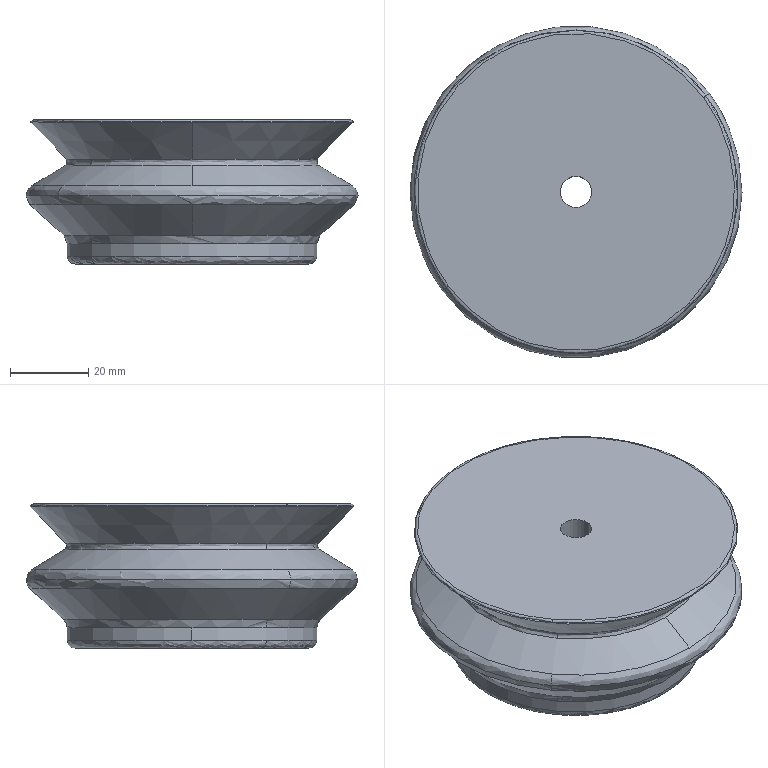Part | SolidWorks | features BaseBody 1 | 1 solid | 26 faces | box 85.101 x 85.101 x 37 mm | volume 155072 mm3 | spline 12 | cone 8 | cylinder 4 | plane 2 | commonest cylinder face diameters 8 x2 64 x2